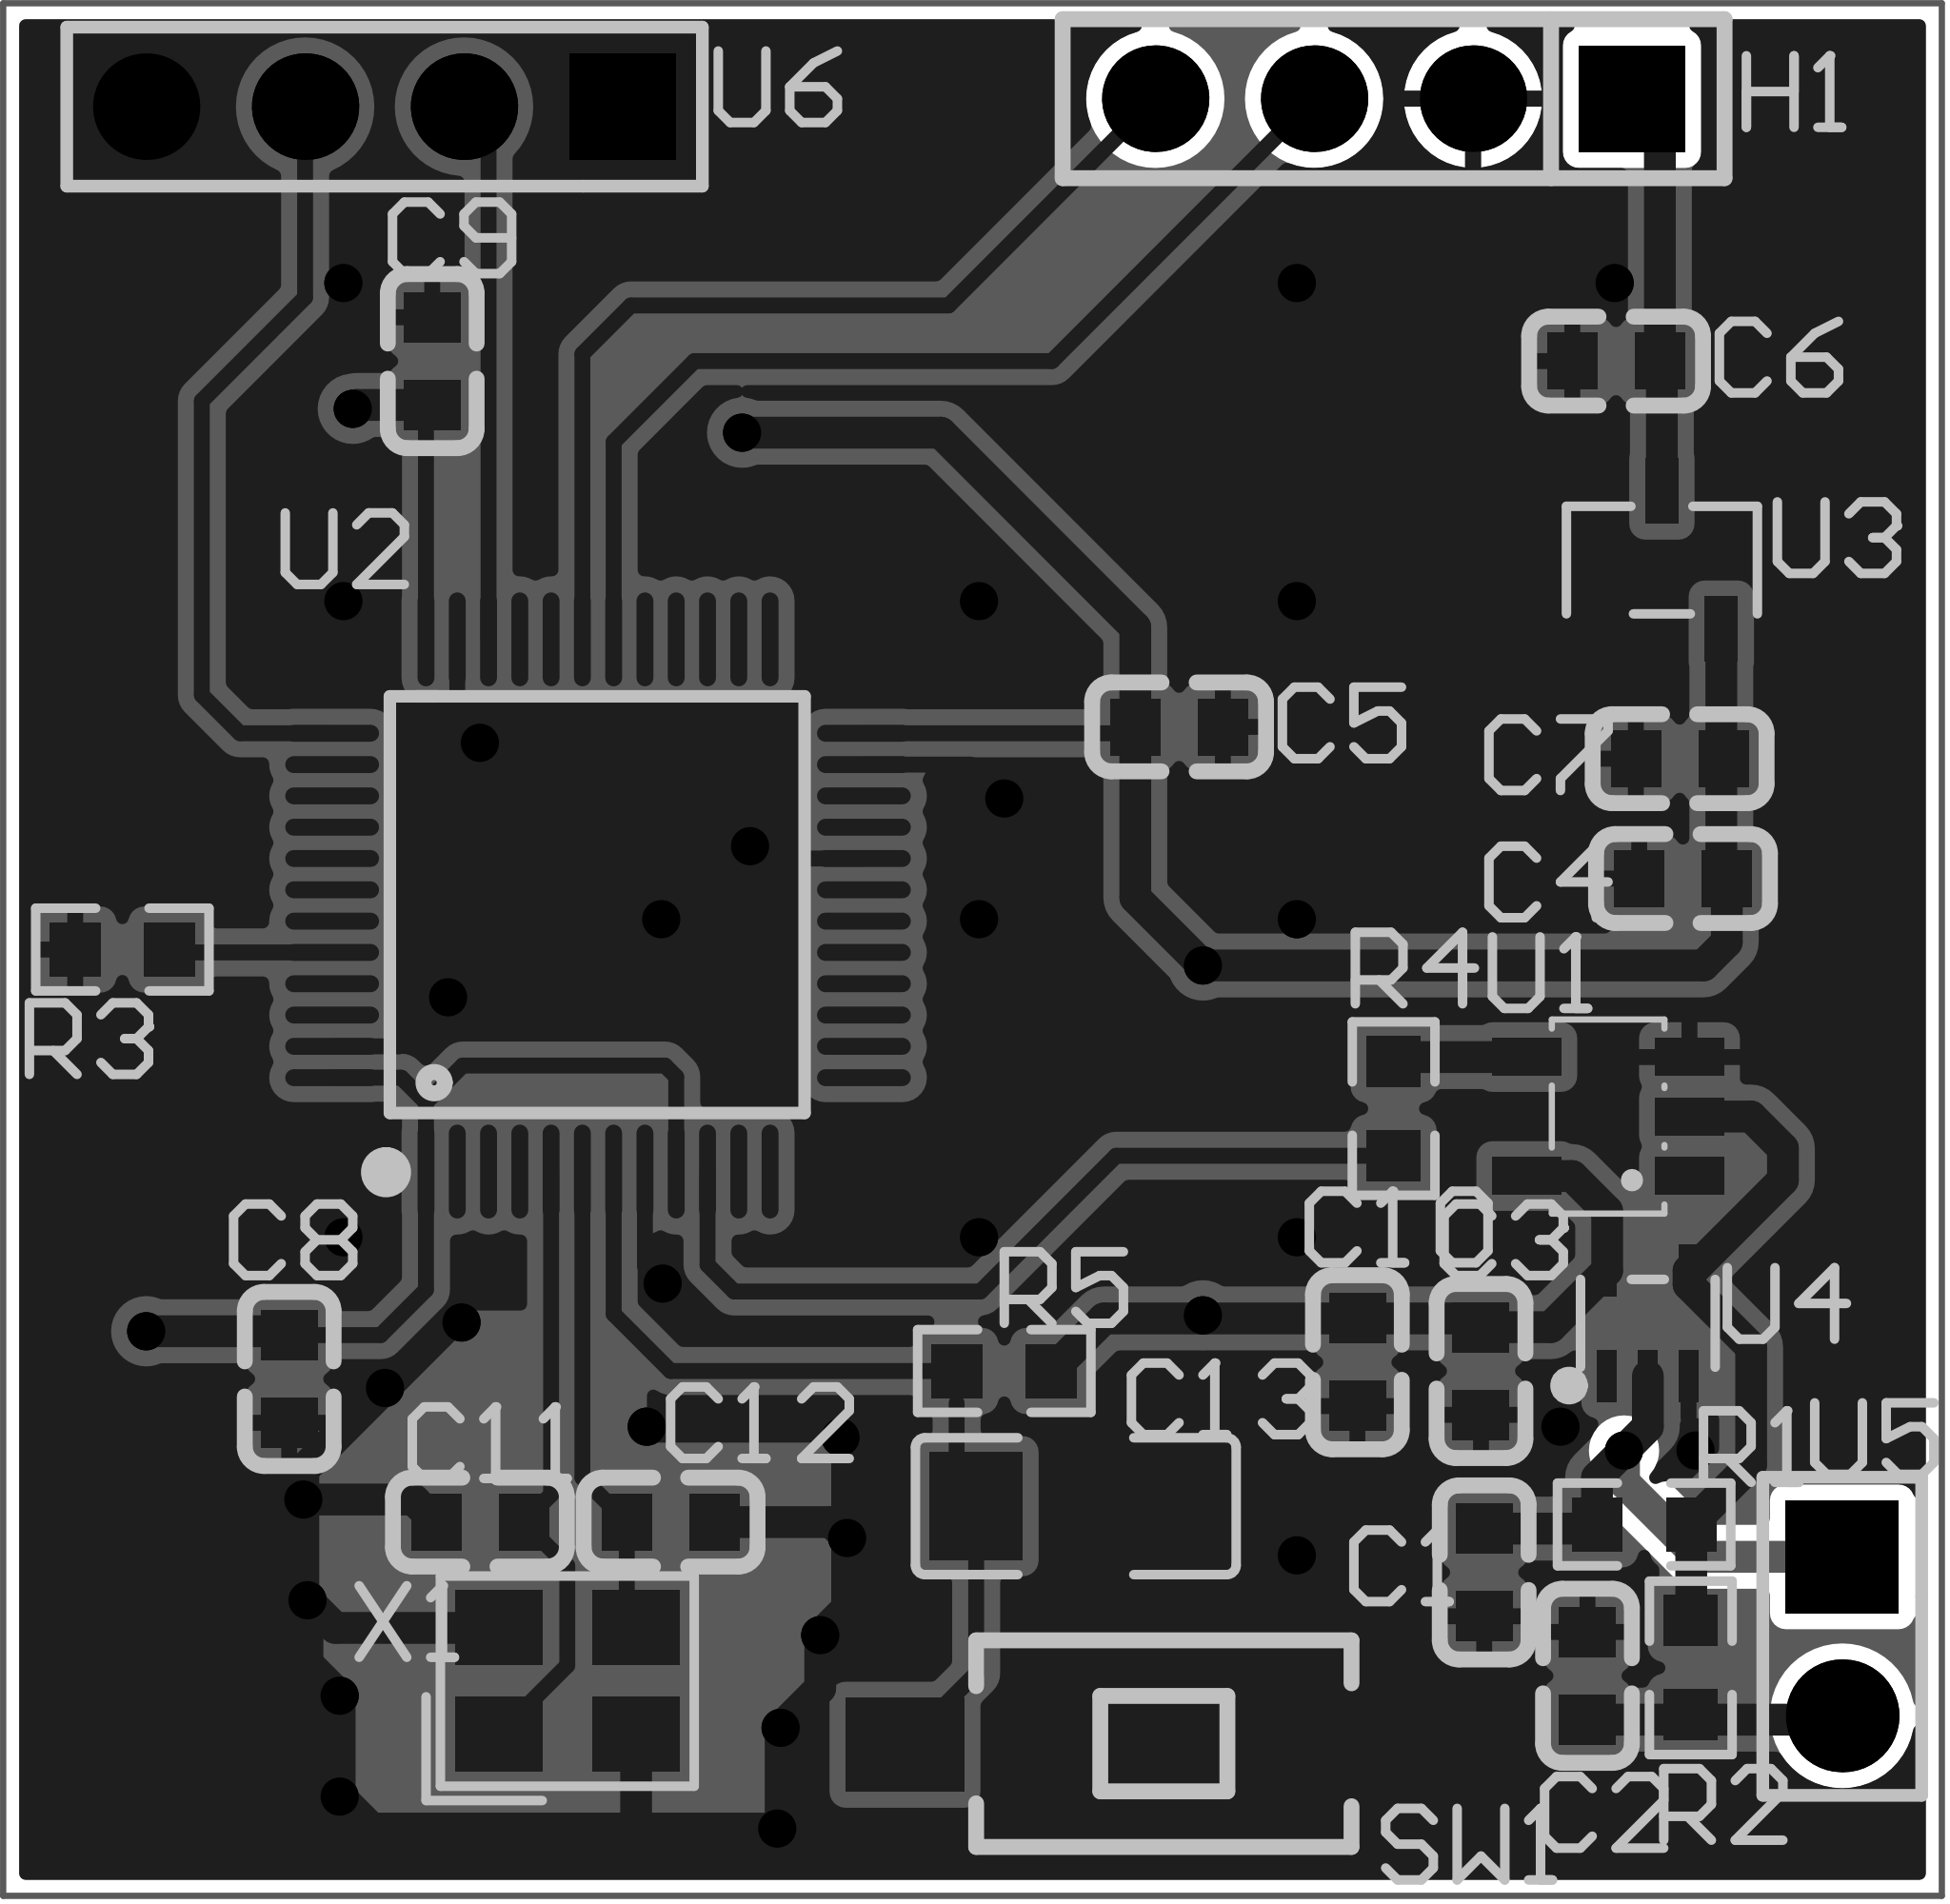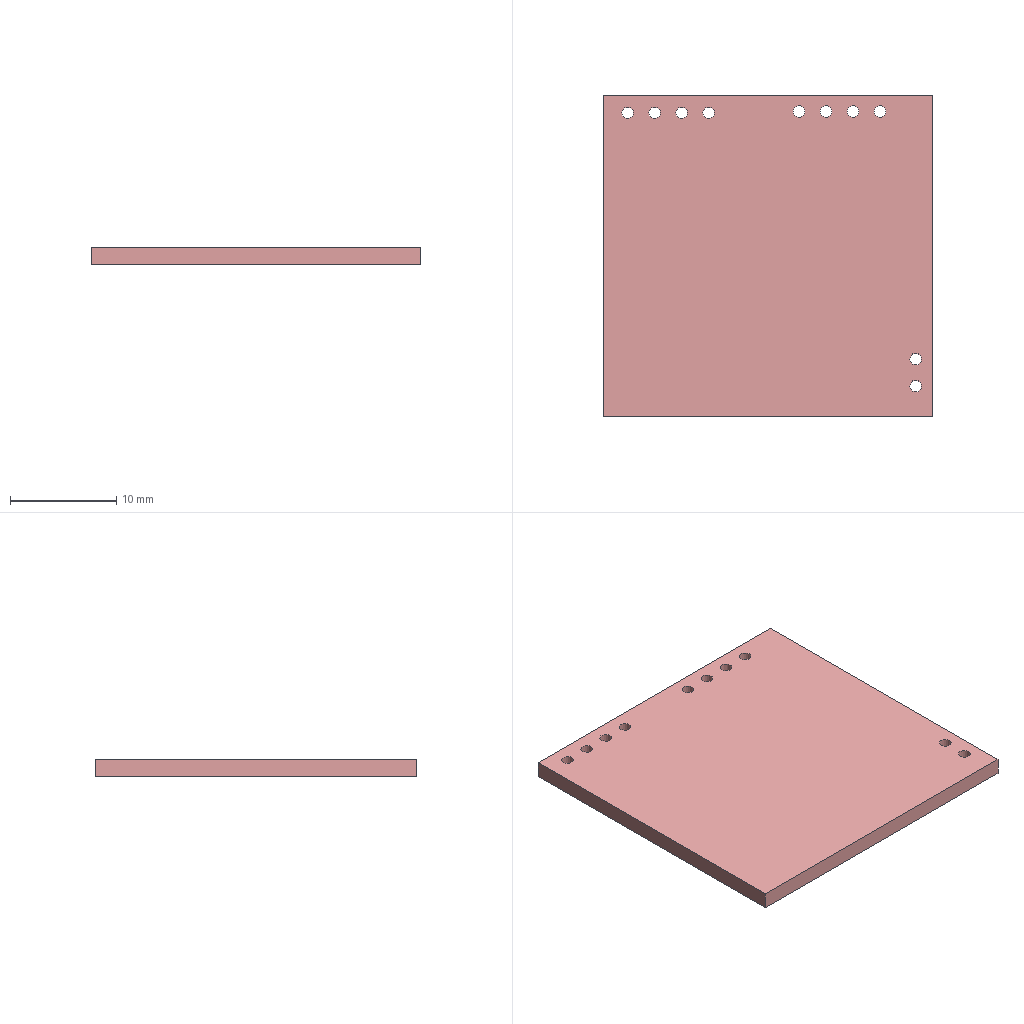Circuit board layout | Altium Designer | box 31 x 30.2 x 1.6 mm
Layer stack:
# Altium Designer layer stack of  (unit mm; dielectric type: 0 none, 1 core, 2 prepreg, 3 surface material)
index,name,kind,layer,copper_thickness_mm,dielectric_type,dielectric_thickness_mm,dielectric_material,dielectric_constant
0,Top Paste Mask Layer,other,,,,,,
1,Top Silkscreen Layer,other,,,,,,
2,Top Solder Mask Layer,dielectric,,,3,0.01,,3.3
3,Top Layer,copper,Top Layer,0.035,,,,
4,Dielectric1,dielectric,,,3,1.51,FR4,4.5
5,Bottom Layer,copper,Bottom Layer,0.035,,,,
6,Bottom Solder Mask Layer,dielectric,,,3,0.01,,3.3
7,Bottom Silkscreen Layer,other,,,,,,
8,Bottom Paste Mask Layer,other,,,,,,
# drill layer pairs: low layer,high layer
drill_pair,Top Layer,Bottom Layer
Part placement:
Designator,Comment,Layer,Footprint,Center-X(mm),Center-Y(mm),Rotation
C1,33pF,TopLayer,C0603,103.556,83.905,270
C2,33pF,TopLayer,C0603,105.207,82.254,90
C3,100nF,TopLayer,C0603,103.505,87.122,90
C4,100nF,TopLayer,C0603,106.734,94.987,180
C5,100nF,TopLayer,C0603,98.679,97.409,180
C6,1uF,TopLayer,C0603,105.664,103.251,0
C7,10uF,TopLayer,C0603,106.68,96.901,0
C8,100nF,TopLayer,C0603,84.455,86.995,90
C9,100nF,TopLayer,C0603,86.741,103.251,90
C10,100nF,TopLayer,C0603,101.529,87.262,90
C11,20pF,TopLayer,C0603,87.503,84.709,180
C12,20pF,TopLayer,C0603,90.551,84.709,0
H1,2.54-1*4P female,TopLayer,HDR-TH_4P-P2.54-V-F,102.108,107.442,180
R1,1MΩ,TopLayer,R0603,106.112,84.671,0
R2,510Ω,TopLayer,R0603,106.858,82.381,270
R3,10kΩ,TopLayer,R0603,81.788,93.853,180
R4,33Ω,TopLayer,R0603,102.108,91.313,90
U1,SN74LVC1G14DBVR,TopLayer,SOT-23-5_L3.0-W1.7-P0.95-LS2.8-BR,105.537,91.186,0
U2,STM32F103C8T6,TopLayer,LQFP-48_L7.0-W7.0-P0.50-LS9.0-BL,89.391,94.557,0
U3,XC6206P332MR,TopLayer,SOT-23-3_L3.0-W1.7-P0.95-LS2.9-BR,106.396,100.073,270
U4,SN74LVC1GU04DCKR,TopLayer,SC-70-5_L2.1-W1.3-P0.65-LS2.1-BL,106.172,87.884,0
U5,HX PZ2.54-1x2P ZZ,TopLayer,HDR-TH_2P-P2.54-V-M-3,109.279,82.885,270
U6,2541WV-04P,TopLayer,HDR-TH_4P-P2.54-V-M-1,85.979,107.315,180
X1,8MHz,TopLayer,CRYSTAL-SMD_4P-L3.2-W2.5-BL,88.9,82.169,0
C13,100uF,TopLayer,C1206,97.028,84.963,180
R5,1kΩ,TopLayer,R0603,95.885,87.122,0
SW1,TS-1101-C-W,TopLayer,SW-SMD_L6.0-W3.3-LS8.0,98.298,81.153,180
Pad and via stacks:
# Altium Designer via and pad stacks of  (unit mm). Each distinct definition once, with the count of objects using it.
# via: kind,start_layer,end_layer,hole_mm,diameter_mm,mode(0 simple;1 top-mid-bottom;2 full stack),diameter_per_layer,count,example_net
# pad: kind,layer,hole_mm,hole_type(0 round;1 square;2 slot),plating,top_size,top_shape(1 round;2 rect;3 octagon;9 rounded rect),mid_size,bottom_size,mode,footprint,size_per_layer,count,example
pad,Top Layer,0,0,plated,0.8x0.9,2,0.8x0.9,0.8x0.9,0,C0603,,24,C1.2
pad,Top Layer,0,0,plated,0.8065x0.864,2,0.8065x0.864,0.8065x0.864,0,R0603,,10,R1.2
pad,Top Layer,0,0,plated,1.1x0.6,2,1.1x0.6,1.1x0.6,0,SOT-23-5_L3.0-W1.7-P0.95-LS2.8-BR,,5,U1.5
pad,Top Layer,0,0,plated,0.27x1.5,1,0.27x1.5,0.27x1.5,0,LQFP-48_L7.0-W7.0-P0.50-LS9.0-BL,,24,U2.1
pad,Top Layer,0,0,plated,1.5x0.27,1,1.5x0.27,1.5x0.27,0,LQFP-48_L7.0-W7.0-P0.50-LS9.0-BL,,24,U2.13
pad,Top Layer,0,0,plated,1.038x0.532,2,1.038x0.532,1.038x0.532,0,SOT-23-3_L3.0-W1.7-P0.95-LS2.9-BR,,3,U3.1
pad,Top Layer,0,0,plated,0.315x0.835,2,0.315x0.835,0.315x0.835,0,SC-70-5_L2.1-W1.3-P0.65-LS2.1-BL,,5,U4.1
pad,Top Layer,0,0,plated,1.4x1.2,2,1.4x1.2,1.4x1.2,0,CRYSTAL-SMD_4P-L3.2-W2.5-BL,,4,X1.1
pad,Top Layer,0,0,plated,1.485x1.728,2,1.485x1.728,1.485x1.728,0,C1206,,2,C13.2
pad,Top Layer,0,0,plated,1.9x1.5,2,1.9x1.5,1.9x1.5,0,SW-SMD_L6.0-W3.3-LS8.0,,2,SW1.1
pad,Multi-Layer,1.1,0,plated,1.7x1.7,2,1.7x1.7,1.7x1.7,0,HDR-TH_4P-P2.54-V-F,,1,H1.1
pad,Multi-Layer,1.1,0,plated,1.7x1.7,1,1.7x1.7,1.7x1.7,0,HDR-TH_4P-P2.54-V-F,,3,H1.2
pad,Multi-Layer,1.1,0,plated,1.8x1.8,2,1.8x1.8,1.8x1.8,0,HDR-TH_2P-P2.54-V-M-3,,1,U5.1
pad,Multi-Layer,1.1,0,plated,1.8x1.8,1,1.8x1.8,1.8x1.8,0,HDR-TH_2P-P2.54-V-M-3,,1,U5.2
pad,Multi-Layer,1.1,0,plated,1.7x1.7,2,1.7x1.7,1.7x1.7,0,HDR-TH_4P-P2.54-V-M-1,,1,U6.1
pad,Multi-Layer,1.1,0,plated,1.7x1.7,1,1.7x1.7,1.7x1.7,0,HDR-TH_4P-P2.54-V-M-1,,3,U6.2
via,Top Layer,Bottom Layer,0.3048,0.61,0,,38,$1N30
Copper pours:
name,layer,net,type(0 solid;1 hatched;2 none)
Top Layer-GND,Top Layer,GND,0
Bottom Layer-GND,Bottom Layer,GND,0